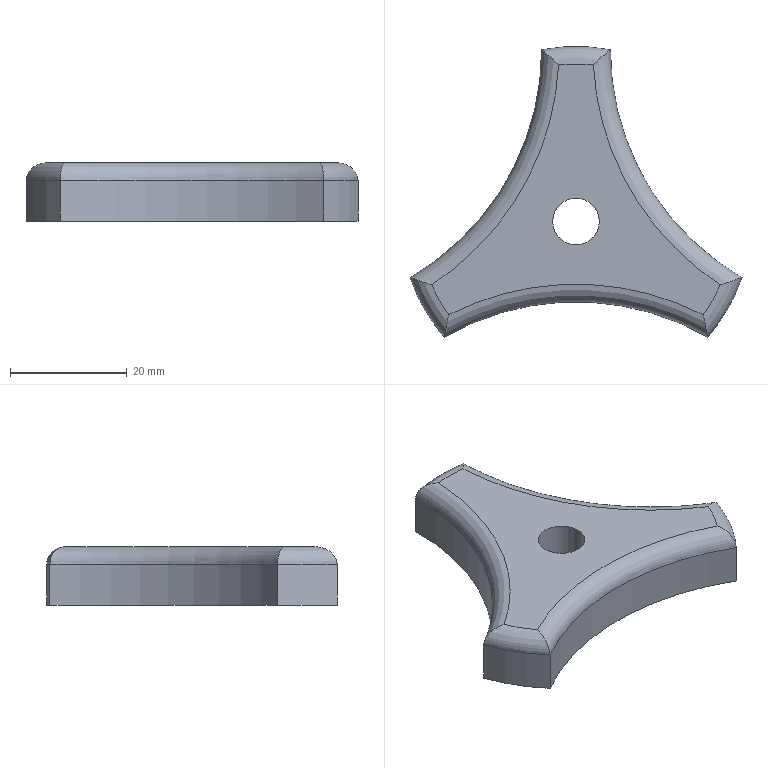Part | STEP file | Superstructure_1 | 1 solid | 15 faces | box 56.861 x 49.792 x 10 mm | volume 12371 mm3 | cylinder 7 | torus 6 | plane 2 | commonest cylinder face diameters 60 x3 90 x3 8 x1